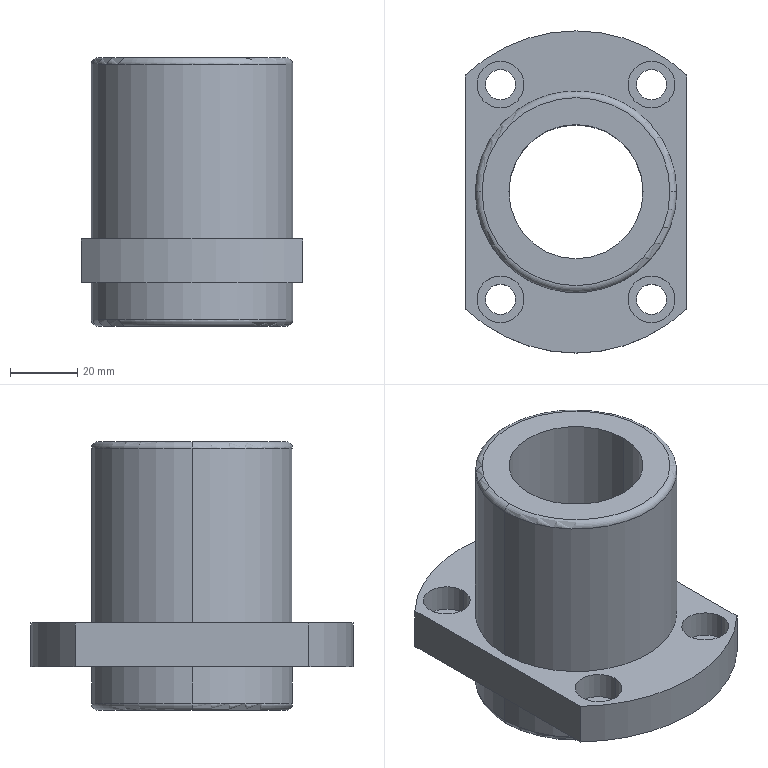Part | SolidWorks | features RevCut 4, ICE 1, LockFeature 1, Revolution 1 | 1 solid | 38 faces | box 66 x 96 x 80 mm | volume 157671 mm3 | cylinder 24 | plane 10 | torus 4 | commonest cylinder face diameters 9 x8 14 x8 60 x4 40 x2 96 x2
STEP:
#1=CARTESIAN_POINT('',(15.5,-32.,4.9));
#2=VERTEX_POINT('',#1);
#3=CARTESIAN_POINT('',(29.5,-32.,4.9));
#4=VERTEX_POINT('',#3);
#5=CARTESIAN_POINT('',(22.5,-32.,4.9));
#6=DIRECTION('',(0.,0.,1.));
#7=DIRECTION('',(1.,0.,0.));
#8=AXIS2_PLACEMENT_3D('',#5,#6,#7);
#9=CIRCLE('',#8,7.);
#10=EDGE_CURVE('',#2,#4,#9,.T.);
#11=ORIENTED_EDGE('',*,*,#10,.F.);
#12=CARTESIAN_POINT('',(15.5,-32.,13.));
#13=VERTEX_POINT('',#12);
#14=CARTESIAN_POINT('',(15.5,-32.,13.));
#15=DIRECTION('',(0.,0.,1.));
#16=VECTOR('',#15,1000.);
#17=LINE('',#14,#16);
#18=EDGE_CURVE('',#2,#13,#17,.T.);
#19=ORIENTED_EDGE('',*,*,#18,.T.);
#20=CARTESIAN_POINT('',(29.5,-32.,13.));
#21=VERTEX_POINT('',#20);
#22=CARTESIAN_POINT('',(22.5,-32.,13.));
#23=DIRECTION('',(0.,0.,1.));
#24=DIRECTION('',(1.,0.,0.));
#25=AXIS2_PLACEMENT_3D('',#22,#23,#24);
#26=CIRCLE('',#25,7.);
#27=EDGE_CURVE('',#13,#21,#26,.T.);
#28=ORIENTED_EDGE('',*,*,#27,.T.);
#29=CARTESIAN_POINT('',(29.5,-32.,13.));
#30=DIRECTION('',(0.,0.,1.));
#31=VECTOR('',#30,1000.);
#32=LINE('',#29,#31);
#33=EDGE_CURVE('',#4,#21,#32,.T.);
#34=ORIENTED_EDGE('',*,*,#33,.F.);
#35=EDGE_LOOP('',(#11,#19,#28,#34));
#36=FACE_OUTER_BOUND('',#35,.T.);
#37=CARTESIAN_POINT('',(22.5,-32.,13.));
#38=DIRECTION('',(0.,0.,1.));
#39=DIRECTION('',(1.,0.,0.));
#40=AXIS2_PLACEMENT_3D('',#37,#38,#39);
#41=CYLINDRICAL_SURFACE('',#40,7.);
#42=ADVANCED_FACE('',(#36),#41,.F.);
#43=CARTESIAN_POINT('',(18.,-32.,0.));
#44=VERTEX_POINT('',#43);
#45=CARTESIAN_POINT('',(27.,-32.,0.));
#46=VERTEX_POINT('',#45);
#47=CARTESIAN_POINT('',(22.5,-32.,0.));
#48=DIRECTION('',(0.,0.,1.));
#49=DIRECTION('',(1.,0.,0.));
#50=AXIS2_PLACEMENT_3D('',#47,#48,#49);
#51=CIRCLE('',#50,4.5);
#52=EDGE_CURVE('',#44,#46,#51,.T.);
#53=ORIENTED_EDGE('',*,*,#52,.F.);
#54=CARTESIAN_POINT('',(18.,-32.,4.9));
#55=VERTEX_POINT('',#54);
#56=CARTESIAN_POINT('',(18.,-32.,13.));
#57=DIRECTION('',(0.,0.,1.));
#58=VECTOR('',#57,1000.);
#59=LINE('',#56,#58);
#60=EDGE_CURVE('',#44,#55,#59,.T.);
#61=ORIENTED_EDGE('',*,*,#60,.T.);
#62=CARTESIAN_POINT('',(27.,-32.,4.9));
#63=VERTEX_POINT('',#62);
#64=CARTESIAN_POINT('',(22.5,-32.,4.9));
#65=DIRECTION('',(0.,0.,1.));
#66=DIRECTION('',(1.,0.,0.));
#67=AXIS2_PLACEMENT_3D('',#64,#65,#66);
#68=CIRCLE('',#67,4.5);
#69=EDGE_CURVE('',#55,#63,#68,.T.);
#70=ORIENTED_EDGE('',*,*,#69,.T.);
#71=CARTESIAN_POINT('',(27.,-32.,13.));
#72=DIRECTION('',(0.,0.,1.));
#73=VECTOR('',#72,1000.);
#74=LINE('',#71,#73);
#75=EDGE_CURVE('',#46,#63,#74,.T.);
#76=ORIENTED_EDGE('',*,*,#75,.F.);
#77=EDGE_LOOP('',(#53,#61,#70,#76));
#78=FACE_OUTER_BOUND('',#77,.T.);
#79=CARTESIAN_POINT('',(22.5,-32.,13.));
#80=DIRECTION('',(0.,0.,1.));
#81=DIRECTION('',(1.,0.,0.));
#82=AXIS2_PLACEMENT_3D('',#79,#80,#81);
#83=CYLINDRICAL_SURFACE('',#82,4.5);
#84=ADVANCED_FACE('',(#78),#83,.F.);
#85=CARTESIAN_POINT('',(27.,32.,4.9));
#86=VERTEX_POINT('',#85);
#87=CARTESIAN_POINT('',(18.,32.,4.9));
#88=VERTEX_POINT('',#87);
#89=CARTESIAN_POINT('',(22.5,32.,4.9));
#90=DIRECTION('',(0.,0.,-1.));
#91=DIRECTION('',(-1.,0.,0.));
#92=AXIS2_PLACEMENT_3D('',#89,#90,#91);
#93=CIRCLE('',#92,4.5);
#94=EDGE_CURVE('',#86,#88,#93,.T.);
#95=ORIENTED_EDGE('',*,*,#94,.F.);
#96=CARTESIAN_POINT('',(27.,32.,0.));
#97=VERTEX_POINT('',#96);
#98=CARTESIAN_POINT('',(27.,32.,0.));
#99=DIRECTION('',(0.,0.,-1.));
#100=VECTOR('',#99,1000.);
#101=LINE('',#98,#100);
#102=EDGE_CURVE('',#86,#97,#101,.T.);
#103=ORIENTED_EDGE('',*,*,#102,.T.);
#104=CARTESIAN_POINT('',(18.,32.,0.));
#105=VERTEX_POINT('',#104);
#106=CARTESIAN_POINT('',(22.5,32.,0.));
#107=DIRECTION('',(0.,0.,-1.));
#108=DIRECTION('',(-1.,0.,0.));
#109=AXIS2_PLACEMENT_3D('',#106,#107,#108);
#110=CIRCLE('',#109,4.5);
#111=EDGE_CURVE('',#97,#105,#110,.T.);
#112=ORIENTED_EDGE('',*,*,#111,.T.);
#113=CARTESIAN_POINT('',(18.,32.,0.));
#114=DIRECTION('',(0.,0.,-1.));
#115=VECTOR('',#114,1000.);
#116=LINE('',#113,#115);
#117=EDGE_CURVE('',#88,#105,#116,.T.);
#118=ORIENTED_EDGE('',*,*,#117,.F.);
#119=EDGE_LOOP('',(#95,#103,#112,#118));
#120=FACE_OUTER_BOUND('',#119,.T.);
#121=CARTESIAN_POINT('',(22.5,32.,0.));
#122=DIRECTION('',(0.,0.,-1.));
#123=DIRECTION('',(-1.,0.,0.));
#124=AXIS2_PLACEMENT_3D('',#121,#122,#123);
#125=CYLINDRICAL_SURFACE('',#124,4.5);
#126=ADVANCED_FACE('',(#120),#125,.F.);
#127=CARTESIAN_POINT('',(29.5,32.,13.));
#128=VERTEX_POINT('',#127);
#129=CARTESIAN_POINT('',(15.5,32.,13.));
#130=VERTEX_POINT('',#129);
#131=CARTESIAN_POINT('',(22.5,32.,13.));
#132=DIRECTION('',(0.,0.,-1.));
#133=DIRECTION('',(-1.,0.,0.));
#134=AXIS2_PLACEMENT_3D('',#131,#132,#133);
#135=CIRCLE('',#134,7.);
#136=EDGE_CURVE('',#128,#130,#135,.T.);
#137=ORIENTED_EDGE('',*,*,#136,.F.);
#138=CARTESIAN_POINT('',(29.5,32.,4.9));
#139=VERTEX_POINT('',#138);
#140=CARTESIAN_POINT('',(29.5,32.,0.));
#141=DIRECTION('',(0.,0.,-1.));
#142=VECTOR('',#141,1000.);
#143=LINE('',#140,#142);
#144=EDGE_CURVE('',#128,#139,#143,.T.);
#145=ORIENTED_EDGE('',*,*,#144,.T.);
#146=CARTESIAN_POINT('',(15.5,32.,4.9));
#147=VERTEX_POINT('',#146);
#148=CARTESIAN_POINT('',(22.5,32.,4.9));
#149=DIRECTION('',(0.,0.,-1.));
#150=DIRECTION('',(-1.,0.,0.));
#151=AXIS2_PLACEMENT_3D('',#148,#149,#150);
#152=CIRCLE('',#151,7.);
#153=EDGE_CURVE('',#139,#147,#152,.T.);
#154=ORIENTED_EDGE('',*,*,#153,.T.);
#155=CARTESIAN_POINT('',(15.5,32.,0.));
#156=DIRECTION('',(0.,0.,-1.));
#157=VECTOR('',#156,1000.);
#158=LINE('',#155,#157);
#159=EDGE_CURVE('',#130,#147,#158,.T.);
#160=ORIENTED_EDGE('',*,*,#159,.F.);
#161=EDGE_LOOP('',(#137,#145,#154,#160));
#162=FACE_OUTER_BOUND('',#161,.T.);
#163=CARTESIAN_POINT('',(22.5,32.,0.));
#164=DIRECTION('',(0.,0.,-1.));
#165=DIRECTION('',(-1.,0.,0.));
#166=AXIS2_PLACEMENT_3D('',#163,#164,#165);
#167=CYLINDRICAL_SURFACE('',#166,7.);
#168=ADVANCED_FACE('',(#162),#167,.F.);
#169=CARTESIAN_POINT('',(-29.5,-32.,4.9));
#170=VERTEX_POINT('',#169);
#171=CARTESIAN_POINT('',(-15.5,-32.,4.9));
#172=VERTEX_POINT('',#171);
#173=CARTESIAN_POINT('',(-22.5,-32.,4.9));
#174=DIRECTION('',(0.,0.,1.));
#175=DIRECTION('',(1.,0.,0.));
#176=AXIS2_PLACEMENT_3D('',#173,#174,#175);
#177=CIRCLE('',#176,7.);
#178=EDGE_CURVE('',#170,#172,#177,.T.);
#179=ORIENTED_EDGE('',*,*,#178,.F.);
#180=CARTESIAN_POINT('',(-29.5,-32.,13.));
#181=VERTEX_POINT('',#180);
#182=CARTESIAN_POINT('',(-29.5,-32.,13.));
#183=DIRECTION('',(0.,0.,1.));
#184=VECTOR('',#183,1000.);
#185=LINE('',#182,#184);
#186=EDGE_CURVE('',#170,#181,#185,.T.);
#187=ORIENTED_EDGE('',*,*,#186,.T.);
#188=CARTESIAN_POINT('',(-15.5,-32.,13.));
#189=VERTEX_POINT('',#188);
#190=CARTESIAN_POINT('',(-22.5,-32.,13.));
#191=DIRECTION('',(0.,0.,1.));
#192=DIRECTION('',(1.,0.,0.));
#193=AXIS2_PLACEMENT_3D('',#190,#191,#192);
#194=CIRCLE('',#193,7.);
#195=EDGE_CURVE('',#181,#189,#194,.T.);
#196=ORIENTED_EDGE('',*,*,#195,.T.);
#197=CARTESIAN_POINT('',(-15.5,-32.,13.));
#198=DIRECTION('',(0.,0.,1.));
#199=VECTOR('',#198,1000.);
#200=LINE('',#197,#199);
#201=EDGE_CURVE('',#172,#189,#200,.T.);
#202=ORIENTED_EDGE('',*,*,#201,.F.);
#203=EDGE_LOOP('',(#179,#187,#196,#202));
#204=FACE_OUTER_BOUND('',#203,.T.);
#205=CARTESIAN_POINT('',(-22.5,-32.,13.));
#206=DIRECTION('',(0.,0.,1.));
#207=DIRECTION('',(1.,0.,0.));
#208=AXIS2_PLACEMENT_3D('',#205,#206,#207);
#209=CYLINDRICAL_SURFACE('',#208,7.);
#210=ADVANCED_FACE('',(#204),#209,.F.);
#211=CARTESIAN_POINT('',(-27.,-32.,0.));
#212=VERTEX_POINT('',#211);
#213=CARTESIAN_POINT('',(-18.,-32.,0.));
#214=VERTEX_POINT('',#213);
#215=CARTESIAN_POINT('',(-22.5,-32.,0.));
#216=DIRECTION('',(0.,0.,1.));
#217=DIRECTION('',(1.,0.,0.));
#218=AXIS2_PLACEMENT_3D('',#215,#216,#217);
#219=CIRCLE('',#218,4.5);
#220=EDGE_CURVE('',#212,#214,#219,.T.);
#221=ORIENTED_EDGE('',*,*,#220,.F.);
#222=CARTESIAN_POINT('',(-27.,-32.,4.9));
#223=VERTEX_POINT('',#222);
#224=CARTESIAN_POINT('',(-27.,-32.,13.));
#225=DIRECTION('',(0.,0.,1.));
#226=VECTOR('',#225,1000.);
#227=LINE('',#224,#226);
#228=EDGE_CURVE('',#212,#223,#227,.T.);
#229=ORIENTED_EDGE('',*,*,#228,.T.);
#230=CARTESIAN_POINT('',(-18.,-32.,4.9));
#231=VERTEX_POINT('',#230);
#232=CARTESIAN_POINT('',(-22.5,-32.,4.9));
#233=DIRECTION('',(0.,0.,1.));
#234=DIRECTION('',(1.,0.,0.));
#235=AXIS2_PLACEMENT_3D('',#232,#233,#234);
#236=CIRCLE('',#235,4.5);
#237=EDGE_CURVE('',#223,#231,#236,.T.);
#238=ORIENTED_EDGE('',*,*,#237,.T.);
#239=CARTESIAN_POINT('',(-18.,-32.,13.));
#240=DIRECTION('',(0.,0.,1.));
#241=VECTOR('',#240,1000.);
#242=LINE('',#239,#241);
#243=EDGE_CURVE('',#214,#231,#242,.T.);
#244=ORIENTED_EDGE('',*,*,#243,.F.);
#245=EDGE_LOOP('',(#221,#229,#238,#244));
#246=FACE_OUTER_BOUND('',#245,.T.);
#247=CARTESIAN_POINT('',(-22.5,-32.,13.));
#248=DIRECTION('',(0.,0.,1.));
#249=DIRECTION('',(1.,0.,0.));
#250=AXIS2_PLACEMENT_3D('',#247,#248,#249);
#251=CYLINDRICAL_SURFACE('',#250,4.5);
#252=ADVANCED_FACE('',(#246),#251,.F.);
#253=CARTESIAN_POINT('',(-18.,32.,4.9));
#254=VERTEX_POINT('',#253);
#255=CARTESIAN_POINT('',(-27.,32.,4.9));
#256=VERTEX_POINT('',#255);
#257=CARTESIAN_POINT('',(-22.5,32.,4.9));
#258=DIRECTION('',(0.,0.,-1.));
#259=DIRECTION('',(-1.,0.,0.));
#260=AXIS2_PLACEMENT_3D('',#257,#258,#259);
#261=CIRCLE('',#260,4.5);
#262=EDGE_CURVE('',#254,#256,#261,.T.);
#263=ORIENTED_EDGE('',*,*,#262,.F.);
#264=CARTESIAN_POINT('',(-18.,32.,0.));
#265=VERTEX_POINT('',#264);
#266=CARTESIAN_POINT('',(-18.,32.,0.));
#267=DIRECTION('',(0.,0.,-1.));
#268=VECTOR('',#267,1000.);
#269=LINE('',#266,#268);
#270=EDGE_CURVE('',#254,#265,#269,.T.);
#271=ORIENTED_EDGE('',*,*,#270,.T.);
#272=CARTESIAN_POINT('',(-27.,32.,0.));
#273=VERTEX_POINT('',#272);
#274=CARTESIAN_POINT('',(-22.5,32.,0.));
#275=DIRECTION('',(0.,0.,-1.));
#276=DIRECTION('',(-1.,0.,0.));
#277=AXIS2_PLACEMENT_3D('',#274,#275,#276);
#278=CIRCLE('',#277,4.5);
#279=EDGE_CURVE('',#265,#273,#278,.T.);
#280=ORIENTED_EDGE('',*,*,#279,.T.);
#281=CARTESIAN_POINT('',(-27.,32.,0.));
#282=DIRECTION('',(0.,0.,-1.));
#283=VECTOR('',#282,1000.);
#284=LINE('',#281,#283);
#285=EDGE_CURVE('',#256,#273,#284,.T.);
#286=ORIENTED_EDGE('',*,*,#285,.F.);
#287=EDGE_LOOP('',(#263,#271,#280,#286));
#288=FACE_OUTER_BOUND('',#287,.T.);
#289=CARTESIAN_POINT('',(-22.5,32.,0.));
#290=DIRECTION('',(0.,0.,-1.));
#291=DIRECTION('',(-1.,0.,0.));
#292=AXIS2_PLACEMENT_3D('',#289,#290,#291);
#293=CYLINDRICAL_SURFACE('',#292,4.5);
#294=ADVANCED_FACE('',(#288),#293,.F.);
#295=CARTESIAN_POINT('',(-15.5,32.,13.));
#296=VERTEX_POINT('',#295);
#297=CARTESIAN_POINT('',(-29.5,32.,13.));
#298=VERTEX_POINT('',#297);
#299=CARTESIAN_POINT('',(-22.5,32.,13.));
#300=DIRECTION('',(0.,0.,-1.));
#301=DIRECTION('',(-1.,0.,0.));
#302=AXIS2_PLACEMENT_3D('',#299,#300,#301);
#303=CIRCLE('',#302,7.);
#304=EDGE_CURVE('',#296,#298,#303,.T.);
#305=ORIENTED_EDGE('',*,*,#304,.F.);
#306=CARTESIAN_POINT('',(-15.5,32.,4.9));
#307=VERTEX_POINT('',#306);
#308=CARTESIAN_POINT('',(-15.5,32.,0.));
#309=DIRECTION('',(0.,0.,-1.));
#310=VECTOR('',#309,1000.);
#311=LINE('',#308,#310);
#312=EDGE_CURVE('',#296,#307,#311,.T.);
#313=ORIENTED_EDGE('',*,*,#312,.T.);
#314=CARTESIAN_POINT('',(-29.5,32.,4.9));
#315=VERTEX_POINT('',#314);
#316=CARTESIAN_POINT('',(-22.5,32.,4.9));
#317=DIRECTION('',(0.,0.,-1.));
#318=DIRECTION('',(-1.,0.,0.));
#319=AXIS2_PLACEMENT_3D('',#316,#317,#318);
#320=CIRCLE('',#319,7.);
#321=EDGE_CURVE('',#307,#315,#320,.T.);
#322=ORIENTED_EDGE('',*,*,#321,.T.);
#323=CARTESIAN_POINT('',(-29.5,32.,0.));
#324=DIRECTION('',(0.,0.,-1.));
#325=VECTOR('',#324,1000.);
#326=LINE('',#323,#325);
#327=EDGE_CURVE('',#298,#315,#326,.T.);
#328=ORIENTED_EDGE('',*,*,#327,.F.);
#329=EDGE_LOOP('',(#305,#313,#322,#328));
#330=FACE_OUTER_BOUND('',#329,.T.);
#331=CARTESIAN_POINT('',(-22.5,32.,0.));
#332=DIRECTION('',(0.,0.,-1.));
#333=DIRECTION('',(-1.,0.,0.));
#334=AXIS2_PLACEMENT_3D('',#331,#332,#333);
#335=CYLINDRICAL_SURFACE('',#334,7.);
#336=ADVANCED_FACE('',(#330),#335,.F.);
#337=CARTESIAN_POINT('',(-30.,0.,65.));
#338=VERTEX_POINT('',#337);
#339=CARTESIAN_POINT('',(30.,0.,65.));
#340=VERTEX_POINT('',#339);
#341=CARTESIAN_POINT('',(0.,0.,65.));
#342=DIRECTION('',(0.,0.,-1.));
#343=DIRECTION('',(-1.,0.,0.));
#344=AXIS2_PLACEMENT_3D('',#341,#342,#343);
#345=CIRCLE('',#344,30.);
#346=EDGE_CURVE('',#338,#340,#345,.T.);
#347=ORIENTED_EDGE('',*,*,#346,.T.);
#348=CARTESIAN_POINT('',(30.,0.,13.));
#349=VERTEX_POINT('',#348);
#350=CARTESIAN_POINT('',(30.,0.,-13.));
#351=DIRECTION('',(0.,0.,-1.));
#352=VECTOR('',#351,1000.);
#353=LINE('',#350,#352);
#354=EDGE_CURVE('',#340,#349,#353,.T.);
#355=ORIENTED_EDGE('',*,*,#354,.T.);
#356=CARTESIAN_POINT('',(-30.,0.,13.));
#357=VERTEX_POINT('',#356);
#358=CARTESIAN_POINT('',(0.,0.,13.));
#359=DIRECTION('',(0.,0.,-1.));
#360=DIRECTION('',(1.,0.,0.));
#361=AXIS2_PLACEMENT_3D('',#358,#359,#360);
#362=CIRCLE('',#361,30.);
#363=EDGE_CURVE('',#357,#349,#362,.T.);
#364=ORIENTED_EDGE('',*,*,#363,.F.);
#365=CARTESIAN_POINT('',(-30.,0.,-13.));
#366=DIRECTION('',(0.,0.,-1.));
#367=VECTOR('',#366,1000.);
#368=LINE('',#365,#367);
#369=EDGE_CURVE('',#338,#357,#368,.T.);
#370=ORIENTED_EDGE('',*,*,#369,.F.);
#371=EDGE_LOOP('',(#347,#355,#364,#370));
#372=FACE_OUTER_BOUND('',#371,.T.);
#373=CARTESIAN_POINT('',(0.,0.,-13.));
#374=DIRECTION('',(0.,0.,-1.));
#375=DIRECTION('',(-1.,0.,0.));
#376=AXIS2_PLACEMENT_3D('',#373,#374,#375);
#377=CYLINDRICAL_SURFACE('',#376,30.);
#378=ADVANCED_FACE('',(#372),#377,.T.);
#379=CARTESIAN_POINT('',(-30.,0.,-11.));
#380=VERTEX_POINT('',#379);
#381=CARTESIAN_POINT('',(30.,0.,-11.));
#382=VERTEX_POINT('',#381);
#383=CARTESIAN_POINT('',(0.,0.,-11.));
#384=DIRECTION('',(0.,0.,-1.));
#385=DIRECTION('',(-1.,0.,0.));
#386=AXIS2_PLACEMENT_3D('',#383,#384,#385);
#387=CIRCLE('',#386,30.);
#388=EDGE_CURVE('',#380,#382,#387,.T.);
#389=ORIENTED_EDGE('',*,*,#388,.T.);
#390=CARTESIAN_POINT('',(28.,0.,-13.));
#391=VERTEX_POINT('',#390);
#392=CARTESIAN_POINT('',(28.,0.,-11.));
#393=DIRECTION('',(0.,1.,0.));
#394=DIRECTION('',(-1.,0.,0.));
#395=AXIS2_PLACEMENT_3D('',#392,#393,#394);
#396=CIRCLE('',#395,2.);
#397=EDGE_CURVE('',#382,#391,#396,.T.);
#398=ORIENTED_EDGE('',*,*,#397,.T.);
#399=CARTESIAN_POINT('',(-28.,0.,-13.));
#400=VERTEX_POINT('',#399);
#401=CARTESIAN_POINT('',(0.,0.,-13.));
#402=DIRECTION('',(0.,0.,-1.));
#403=DIRECTION('',(-1.,0.,0.));
#404=AXIS2_PLACEMENT_3D('',#401,#402,#403);
#405=CIRCLE('',#404,28.);
#406=EDGE_CURVE('',#400,#391,#405,.T.);
#407=ORIENTED_EDGE('',*,*,#406,.F.);
#408=CARTESIAN_POINT('',(-28.,0.,-11.));
#409=DIRECTION('',(0.,-1.,0.));
#410=DIRECTION('',(0.,0.,-1.));
#411=AXIS2_PLACEMENT_3D('',#408,#409,#410);
#412=CIRCLE('',#411,2.);
#413=EDGE_CURVE('',#380,#400,#412,.T.);
#414=ORIENTED_EDGE('',*,*,#413,.F.);
#415=EDGE_LOOP('',(#389,#398,#407,#414));
#416=FACE_OUTER_BOUND('',#415,.T.);
#417=CARTESIAN_POINT('',(0.,0.,-11.));
#418=DIRECTION('',(0.,0.,-1.));
#419=DIRECTION('',(-1.,0.,0.));
#420=AXIS2_PLACEMENT_3D('',#417,#418,#419);
#421=TOROIDAL_SURFACE('',#420,28.,2.);
#422=ADVANCED_FACE('',(#416),#421,.T.);
#423=CARTESIAN_POINT('',(20.,0.,67.));
#424=VERTEX_POINT('',#423);
#425=CARTESIAN_POINT('',(-20.,0.,67.));
#426=VERTEX_POINT('',#425);
#427=CARTESIAN_POINT('',(0.,0.,67.));
#428=DIRECTION('',(0.,0.,-1.));
#429=DIRECTION('',(-1.,0.,0.));
#430=AXIS2_PLACEMENT_3D('',#427,#428,#429);
#431=CIRCLE('',#430,20.);
#432=EDGE_CURVE('',#424,#426,#431,.T.);
#433=ORIENTED_EDGE('',*,*,#432,.F.);
#434=CARTESIAN_POINT('',(20.,0.,-13.));
#435=VERTEX_POINT('',#434);
#436=CARTESIAN_POINT('',(20.,0.,-13.));
#437=DIRECTION('',(0.,0.,-1.));
#438=VECTOR('',#437,1000.);
#439=LINE('',#436,#438);
#440=EDGE_CURVE('',#424,#435,#439,.T.);
#441=ORIENTED_EDGE('',*,*,#440,.T.);
#442=CARTESIAN_POINT('',(-20.,0.,-13.));
#443=VERTEX_POINT('',#442);
#444=CARTESIAN_POINT('',(0.,0.,-13.));
#445=DIRECTION('',(0.,0.,-1.));
#446=DIRECTION('',(-1.,0.,0.));
#447=AXIS2_PLACEMENT_3D('',#444,#445,#446);
#448=CIRCLE('',#447,20.);
#449=EDGE_CURVE('',#435,#443,#448,.T.);
#450=ORIENTED_EDGE('',*,*,#449,.T.);
#451=CARTESIAN_POINT('',(-20.,0.,-13.));
#452=DIRECTION('',(0.,0.,-1.));
#453=VECTOR('',#452,1000.);
#454=LINE('',#451,#453);
#455=EDGE_CURVE('',#426,#443,#454,.T.);
#456=ORIENTED_EDGE('',*,*,#455,.F.);
#457=EDGE_LOOP('',(#433,#441,#450,#456));
#458=FACE_OUTER_BOUND('',#457,.T.);
#459=CARTESIAN_POINT('',(0.,0.,-13.));
#460=DIRECTION('',(0.,0.,-1.));
#461=DIRECTION('',(-1.,0.,0.));
#462=AXIS2_PLACEMENT_3D('',#459,#460,#461);
#463=CYLINDRICAL_SURFACE('',#462,20.);
#464=ADVANCED_FACE('',(#458),#463,.F.);
#465=CARTESIAN_POINT('',(-28.,0.,67.));
#466=VERTEX_POINT('',#465);
#467=CARTESIAN_POINT('',(28.,0.,67.));
#468=VERTEX_POINT('',#467);
#469=CARTESIAN_POINT('',(0.,0.,67.));
#470=DIRECTION('',(0.,0.,-1.));
#471=DIRECTION('',(-1.,0.,0.));
#472=AXIS2_PLACEMENT_3D('',#469,#470,#471);
#473=CIRCLE('',#472,28.);
#474=EDGE_CURVE('',#466,#468,#473,.T.);
#475=ORIENTED_EDGE('',*,*,#474,.T.);
#476=CARTESIAN_POINT('',(28.,0.,65.));
#477=DIRECTION('',(0.,1.,0.));
#478=DIRECTION('',(-1.,0.,0.));
#479=AXIS2_PLACEMENT_3D('',#476,#477,#478);
#480=CIRCLE('',#479,2.);
#481=EDGE_CURVE('',#468,#340,#480,.T.);
#482=ORIENTED_EDGE('',*,*,#481,.T.);
#483=ORIENTED_EDGE('',*,*,#346,.F.);
#484=CARTESIAN_POINT('',(-28.,0.,65.));
#485=DIRECTION('',(0.,-1.,0.));
#486=DIRECTION('',(0.,0.,-1.));
#487=AXIS2_PLACEMENT_3D('',#484,#485,#486);
#488=CIRCLE('',#487,2.);
#489=EDGE_CURVE('',#466,#338,#488,.T.);
#490=ORIENTED_EDGE('',*,*,#489,.F.);
#491=EDGE_LOOP('',(#475,#482,#483,#490));
#492=FACE_OUTER_BOUND('',#491,.T.);
#493=CARTESIAN_POINT('',(0.,0.,65.));
#494=DIRECTION('',(0.,0.,-1.));
#495=DIRECTION('',(-1.,0.,0.));
#496=AXIS2_PLACEMENT_3D('',#493,#494,#495);
#497=TOROIDAL_SURFACE('',#496,28.,2.);
#498=ADVANCED_FACE('',(#492),#497,.T.);
#499=CARTESIAN_POINT('',(30.,0.,0.));
#500=VERTEX_POINT('',#499);
#501=CARTESIAN_POINT('',(-30.,0.,0.));
#502=VERTEX_POINT('',#501);
#503=CARTESIAN_POINT('',(0.,0.,0.));
#504=DIRECTION('',(0.,0.,1.));
#505=DIRECTION('',(1.,0.,0.));
#506=AXIS2_PLACEMENT_3D('',#503,#504,#505);
#507=CIRCLE('',#506,30.);
#508=EDGE_CURVE('',#500,#502,#507,.T.);
#509=ORIENTED_EDGE('',*,*,#508,.F.);
#510=CARTESIAN_POINT('',(30.,0.,-13.));
#511=DIRECTION('',(0.,0.,-1.));
#512=VECTOR('',#511,1000.);
#513=LINE('',#510,#512);
#514=EDGE_CURVE('',#500,#382,#513,.T.);
#515=ORIENTED_EDGE('',*,*,#514,.T.);
#516=ORIENTED_EDGE('',*,*,#388,.F.);
#517=CARTESIAN_POINT('',(-30.,0.,-13.));
#518=DIRECTION('',(0.,0.,-1.));
#519=VECTOR('',#518,1000.);
#520=LINE('',#517,#519);
#521=EDGE_CURVE('',#502,#380,#520,.T.);
#522=ORIENTED_EDGE('',*,*,#521,.F.);
#523=EDGE_LOOP('',(#509,#515,#516,#522));
#524=FACE_OUTER_BOUND('',#523,.T.);
#525=CARTESIAN_POINT('',(0.,0.,-13.));
#526=DIRECTION('',(0.,0.,-1.));
#527=DIRECTION('',(-1.,0.,0.));
#528=AXIS2_PLACEMENT_3D('',#525,#526,#527);
#529=CYLINDRICAL_SURFACE('',#528,30.);
#530=ADVANCED_FACE('',(#524),#529,.T.);
#531=ORIENTED_EDGE('',*,*,#514,.F.);
#532=CARTESIAN_POINT('',(0.,0.,0.));
#533=DIRECTION('',(0.,0.,1.));
#534=DIRECTION('',(1.,0.,0.));
#535=AXIS2_PLACEMENT_3D('',#532,#533,#534);
#536=CIRCLE('',#535,30.);
#537=EDGE_CURVE('',#502,#500,#536,.T.);
#538=ORIENTED_EDGE('',*,*,#537,.F.);
#539=ORIENTED_EDGE('',*,*,#521,.T.);
#540=CARTESIAN_POINT('',(0.,0.,-11.));
#541=DIRECTION('',(0.,0.,-1.));
#542=DIRECTION('',(-1.,0.,0.));
#543=AXIS2_PLACEMENT_3D('',#540,#541,#542);
#544=CIRCLE('',#543,30.);
#545=EDGE_CURVE('',#382,#380,#544,.T.);
#546=ORIENTED_EDGE('',*,*,#545,.F.);
#547=EDGE_LOOP('',(#531,#538,#539,#546));
#548=FACE_OUTER_BOUND('',#547,.T.);
#549=CARTESIAN_POINT('',(0.,0.,-13.));
#550=DIRECTION('',(0.,0.,-1.));
#551=DIRECTION('',(-1.,0.,0.));
#552=AXIS2_PLACEMENT_3D('',#549,#550,#551);
#553=CYLINDRICAL_SURFACE('',#552,30.);
#554=ADVANCED_FACE('',(#548),#553,.T.);
#555=ORIENTED_EDGE('',*,*,#481,.F.);
#556=CARTESIAN_POINT('',(0.,0.,67.));
#557=DIRECTION('',(0.,0.,-1.));
#558=DIRECTION('',(-1.,0.,0.));
#559=AXIS2_PLACEMENT_3D('',#556,#557,#558);
#560=CIRCLE('',#559,28.);
#561=EDGE_CURVE('',#468,#466,#560,.T.);
#562=ORIENTED_EDGE('',*,*,#561,.T.);
#563=ORIENTED_EDGE('',*,*,#489,.T.);
#564=CARTESIAN_POINT('',(0.,0.,65.));
#565=DIRECTION('',(0.,0.,-1.));
#566=DIRECTION('',(-1.,0.,0.));
#567=AXIS2_PLACEMENT_3D('',#564,#565,#566);
#568=CIRCLE('',#567,30.);
#569=EDGE_CURVE('',#340,#338,#568,.T.);
#570=ORIENTED_EDGE('',*,*,#569,.F.);
#571=EDGE_LOOP('',(#555,#562,#563,#570));
#572=FACE_OUTER_BOUND('',#571,.T.);
#573=CARTESIAN_POINT('',(0.,0.,65.));
#574=DIRECTION('',(0.,0.,-1.));
#575=DIRECTION('',(-1.,0.,0.));
#576=AXIS2_PLACEMENT_3D('',#573,#574,#575);
#577=TOROIDAL_SURFACE('',#576,28.,2.);
#578=ADVANCED_FACE('',(#572),#577,.T.);
#579=CARTESIAN_POINT('',(0.,0.,67.));
#580=DIRECTION('',(0.,0.,-1.));
#581=DIRECTION('',(-1.,0.,0.));
#582=AXIS2_PLACEMENT_3D('',#579,#580,#581);
#583=CIRCLE('',#582,20.);
#584=EDGE_CURVE('',#426,#424,#583,.T.);
#585=ORIENTED_EDGE('',*,*,#584,.T.);
#586=ORIENTED_EDGE('',*,*,#432,.T.);
#587=EDGE_LOOP('',(#585,#586));
#588=FACE_BOUND('',#587,.T.);
#589=ORIENTED_EDGE('',*,*,#474,.F.);
#590=ORIENTED_EDGE('',*,*,#561,.F.);
#591=EDGE_LOOP('',(#589,#590));
#592=FACE_OUTER_BOUND('',#591,.T.);
#593=CARTESIAN_POINT('',(0.,28.,67.));
#594=DIRECTION('',(0.,0.,1.));
#595=DIRECTION('',(1.,0.,0.));
#596=AXIS2_PLACEMENT_3D('',#593,#594,#595);
#597=PLANE('',#596);
#598=ADVANCED_FACE('',(#588,#592),#597,.T.);
#599=ORIENTED_EDGE('',*,*,#440,.F.);
#600=ORIENTED_EDGE('',*,*,#584,.F.);
#601=ORIENTED_EDGE('',*,*,#455,.T.);
#602=CARTESIAN_POINT('',(0.,0.,-13.));
#603=DIRECTION('',(0.,0.,-1.));
#604=DIRECTION('',(-1.,0.,0.));
#605=AXIS2_PLACEMENT_3D('',#602,#603,#604);
#606=CIRCLE('',#605,20.);
#607=EDGE_CURVE('',#443,#435,#606,.T.);
#608=ORIENTED_EDGE('',*,*,#607,.T.);
#609=EDGE_LOOP('',(#599,#600,#601,#608));
#610=FACE_OUTER_BOUND('',#609,.T.);
#611=CARTESIAN_POINT('',(0.,0.,-13.));
#612=DIRECTION('',(0.,0.,-1.));
#613=DIRECTION('',(-1.,0.,0.));
#614=AXIS2_PLACEMENT_3D('',#611,#612,#613);
#615=CYLINDRICAL_SURFACE('',#614,20.);
#616=ADVANCED_FACE('',(#610),#615,.F.);
#617=ORIENTED_EDGE('',*,*,#406,.T.);
#618=CARTESIAN_POINT('',(0.,0.,-13.));
#619=DIRECTION('',(0.,0.,-1.));
#620=DIRECTION('',(-1.,0.,0.));
#621=AXIS2_PLACEMENT_3D('',#618,#619,#620);
#622=CIRCLE('',#621,28.);
#623=EDGE_CURVE('',#391,#400,#622,.T.);
#624=ORIENTED_EDGE('',*,*,#623,.T.);
#625=EDGE_LOOP('',(#617,#624));
#626=FACE_OUTER_BOUND('',#625,.T.);
#627=ORIENTED_EDGE('',*,*,#607,.F.);
#628=ORIENTED_EDGE('',*,*,#449,.F.);
#629=EDGE_LOOP('',(#627,#628));
#630=FACE_BOUND('',#629,.T.);
#631=CARTESIAN_POINT('',(0.,20.,-13.));
#632=DIRECTION('',(0.,0.,-1.));
#633=DIRECTION('',(-1.,0.,0.));
#634=AXIS2_PLACEMENT_3D('',#631,#632,#633);
#635=PLANE('',#634);
#636=ADVANCED_FACE('',(#626,#630),#635,.T.);
#637=ORIENTED_EDGE('',*,*,#397,.F.);
#638=ORIENTED_EDGE('',*,*,#545,.T.);
#639=ORIENTED_EDGE('',*,*,#413,.T.);
#640=ORIENTED_EDGE('',*,*,#623,.F.);
#641=EDGE_LOOP('',(#637,#638,#639,#640));
#642=FACE_OUTER_BOUND('',#641,.T.);
#643=CARTESIAN_POINT('',(0.,0.,-11.));
#644=DIRECTION('',(0.,0.,-1.));
#645=DIRECTION('',(-1.,0.,0.));
#646=AXIS2_PLACEMENT_3D('',#643,#644,#645);
#647=TOROIDAL_SURFACE('',#646,28.,2.);
#648=ADVANCED_FACE('',(#642),#647,.T.);
#649=ORIENTED_EDGE('',*,*,#354,.F.);
#650=ORIENTED_EDGE('',*,*,#569,.T.);
#651=ORIENTED_EDGE('',*,*,#369,.T.);
#652=CARTESIAN_POINT('',(0.,0.,13.));
#653=DIRECTION('',(0.,0.,-1.));
#654=DIRECTION('',(1.,0.,0.));
#655=AXIS2_PLACEMENT_3D('',#652,#653,#654);
#656=CIRCLE('',#655,30.);
#657=EDGE_CURVE('',#349,#357,#656,.T.);
#658=ORIENTED_EDGE('',*,*,#657,.F.);
#659=EDGE_LOOP('',(#649,#650,#651,#658));
#660=FACE_OUTER_BOUND('',#659,.T.);
#661=CARTESIAN_POINT('',(0.,0.,-13.));
#662=DIRECTION('',(0.,0.,-1.));
#663=DIRECTION('',(-1.,0.,0.));
#664=AXIS2_PLACEMENT_3D('',#661,#662,#663);
#665=CYLINDRICAL_SURFACE('',#664,30.);
#666=ADVANCED_FACE('',(#660),#665,.T.);
#667=CARTESIAN_POINT('',(22.5,-32.,13.));
#668=DIRECTION('',(0.,0.,1.));
#669=DIRECTION('',(1.,0.,0.));
#670=AXIS2_PLACEMENT_3D('',#667,#668,#669);
#671=CIRCLE('',#670,7.);
#672=EDGE_CURVE('',#21,#13,#671,.T.);
#673=ORIENTED_EDGE('',*,*,#672,.F.);
#674=ORIENTED_EDGE('',*,*,#27,.F.);
#675=EDGE_LOOP('',(#673,#674));
#676=FACE_BOUND('',#675,.T.);
#677=CARTESIAN_POINT('',(22.5,32.,13.));
#678=DIRECTION('',(0.,0.,-1.));
#679=DIRECTION('',(-1.,0.,0.));
#680=AXIS2_PLACEMENT_3D('',#677,#678,#679);
#681=CIRCLE('',#680,7.);
#682=EDGE_CURVE('',#130,#128,#681,.T.);
#683=ORIENTED_EDGE('',*,*,#682,.T.);
#684=ORIENTED_EDGE('',*,*,#136,.T.);
#685=EDGE_LOOP('',(#683,#684));
#686=FACE_BOUND('',#685,.T.);
#687=CARTESIAN_POINT('',(-22.5,-32.,13.));
#688=DIRECTION('',(0.,0.,1.));
#689=DIRECTION('',(1.,0.,0.));
#690=AXIS2_PLACEMENT_3D('',#687,#688,#689);
#691=CIRCLE('',#690,7.);
#692=EDGE_CURVE('',#189,#181,#691,.T.);
#693=ORIENTED_EDGE('',*,*,#692,.F.);
#694=ORIENTED_EDGE('',*,*,#195,.F.);
#695=EDGE_LOOP('',(#693,#694));
#696=FACE_BOUND('',#695,.T.);
#697=CARTESIAN_POINT('',(-22.5,32.,13.));
#698=DIRECTION('',(0.,0.,-1.));
#699=DIRECTION('',(-1.,0.,0.));
#700=AXIS2_PLACEMENT_3D('',#697,#698,#699);
#701=CIRCLE('',#700,7.);
#702=EDGE_CURVE('',#298,#296,#701,.T.);
#703=ORIENTED_EDGE('',*,*,#702,.T.);
#704=ORIENTED_EDGE('',*,*,#304,.T.);
#705=EDGE_LOOP('',(#703,#704));
#706=FACE_BOUND('',#705,.T.);
#707=CARTESIAN_POINT('',(33.,34.857,13.));
#708=VERTEX_POINT('',#707);
#709=CARTESIAN_POINT('',(-33.,34.857,13.));
#710=VERTEX_POINT('',#709);
#711=CARTESIAN_POINT('',(0.,0.,13.));
#712=DIRECTION('',(0.,0.,1.));
#713=DIRECTION('',(1.,0.,0.));
#714=AXIS2_PLACEMENT_3D('',#711,#712,#713);
#715=CIRCLE('',#714,48.);
#716=EDGE_CURVE('',#708,#710,#715,.T.);
#717=ORIENTED_EDGE('',*,*,#716,.T.);
#718=CARTESIAN_POINT('',(-33.,-34.857,13.));
#719=VERTEX_POINT('',#718);
#720=CARTESIAN_POINT('',(-33.,34.857,13.));
#721=DIRECTION('',(0.,-1.,0.));
#722=VECTOR('',#721,1000.);
#723=LINE('',#720,#722);
#724=EDGE_CURVE('',#710,#719,#723,.T.);
#725=ORIENTED_EDGE('',*,*,#724,.T.);
#726=CARTESIAN_POINT('',(33.,-34.857,13.));
#727=VERTEX_POINT('',#726);
#728=CARTESIAN_POINT('',(0.,0.,13.));
#729=DIRECTION('',(0.,0.,1.));
#730=DIRECTION('',(1.,0.,0.));
#731=AXIS2_PLACEMENT_3D('',#728,#729,#730);
#732=CIRCLE('',#731,48.);
#733=EDGE_CURVE('',#719,#727,#732,.T.);
#734=ORIENTED_EDGE('',*,*,#733,.T.);
#735=CARTESIAN_POINT('',(33.,-34.857,13.));
#736=DIRECTION('',(0.,1.,0.));
#737=VECTOR('',#736,1000.);
#738=LINE('',#735,#737);
#739=EDGE_CURVE('',#727,#708,#738,.T.);
#740=ORIENTED_EDGE('',*,*,#739,.T.);
#741=EDGE_LOOP('',(#717,#725,#734,#740));
#742=FACE_OUTER_BOUND('',#741,.T.);
#743=ORIENTED_EDGE('',*,*,#363,.T.);
#744=ORIENTED_EDGE('',*,*,#657,.T.);
#745=EDGE_LOOP('',(#743,#744));
#746=FACE_BOUND('',#745,.T.);
#747=CARTESIAN_POINT('',(0.,0.,13.));
#748=DIRECTION('',(0.,0.,1.));
#749=DIRECTION('',(1.,0.,0.));
#750=AXIS2_PLACEMENT_3D('',#747,#748,#749);
#751=PLANE('',#750);
#752=ADVANCED_FACE('',(#676,#686,#696,#706,#742,#746),#751,.T.);
#753=CARTESIAN_POINT('',(22.5,-32.,0.));
#754=DIRECTION('',(0.,0.,1.));
#755=DIRECTION('',(1.,0.,0.));
#756=AXIS2_PLACEMENT_3D('',#753,#754,#755);
#757=CIRCLE('',#756,4.5);
#758=EDGE_CURVE('',#46,#44,#757,.T.);
#759=ORIENTED_EDGE('',*,*,#758,.T.);
#760=ORIENTED_EDGE('',*,*,#52,.T.);
#761=EDGE_LOOP('',(#759,#760));
#762=FACE_BOUND('',#761,.T.);
#763=CARTESIAN_POINT('',(22.5,32.,0.));
#764=DIRECTION('',(0.,0.,-1.));
#765=DIRECTION('',(-1.,0.,0.));
#766=AXIS2_PLACEMENT_3D('',#763,#764,#765);
#767=CIRCLE('',#766,4.5);
#768=EDGE_CURVE('',#105,#97,#767,.T.);
#769=ORIENTED_EDGE('',*,*,#768,.F.);
#770=ORIENTED_EDGE('',*,*,#111,.F.);
#771=EDGE_LOOP('',(#769,#770));
#772=FACE_BOUND('',#771,.T.);
#773=CARTESIAN_POINT('',(-22.5,-32.,0.));
#774=DIRECTION('',(0.,0.,1.));
#775=DIRECTION('',(1.,0.,0.));
#776=AXIS2_PLACEMENT_3D('',#773,#774,#775);
#777=CIRCLE('',#776,4.5);
#778=EDGE_CURVE('',#214,#212,#777,.T.);
#779=ORIENTED_EDGE('',*,*,#778,.T.);
#780=ORIENTED_EDGE('',*,*,#220,.T.);
#781=EDGE_LOOP('',(#779,#780));
#782=FACE_BOUND('',#781,.T.);
#783=CARTESIAN_POINT('',(-22.5,32.,0.));
#784=DIRECTION('',(0.,0.,-1.));
#785=DIRECTION('',(-1.,0.,0.));
#786=AXIS2_PLACEMENT_3D('',#783,#784,#785);
#787=CIRCLE('',#786,4.5);
#788=EDGE_CURVE('',#273,#265,#787,.T.);
#789=ORIENTED_EDGE('',*,*,#788,.F.);
#790=ORIENTED_EDGE('',*,*,#279,.F.);
#791=EDGE_LOOP('',(#789,#790));
#792=FACE_BOUND('',#791,.T.);
#793=CARTESIAN_POINT('',(33.,34.857,0.));
#794=VERTEX_POINT('',#793);
#795=CARTESIAN_POINT('',(-33.,34.857,0.));
#796=VERTEX_POINT('',#795);
#797=CARTESIAN_POINT('',(0.,0.,0.));
#798=DIRECTION('',(0.,0.,1.));
#799=DIRECTION('',(1.,0.,0.));
#800=AXIS2_PLACEMENT_3D('',#797,#798,#799);
#801=CIRCLE('',#800,48.);
#802=EDGE_CURVE('',#794,#796,#801,.T.);
#803=ORIENTED_EDGE('',*,*,#802,.F.);
#804=CARTESIAN_POINT('',(33.,-34.857,0.));
#805=VERTEX_POINT('',#804);
#806=CARTESIAN_POINT('',(33.,-34.857,0.));
#807=DIRECTION('',(0.,1.,0.));
#808=VECTOR('',#807,1000.);
#809=LINE('',#806,#808);
#810=EDGE_CURVE('',#805,#794,#809,.T.);
#811=ORIENTED_EDGE('',*,*,#810,.F.);
#812=CARTESIAN_POINT('',(-33.,-34.857,0.));
#813=VERTEX_POINT('',#812);
#814=CARTESIAN_POINT('',(0.,0.,0.));
#815=DIRECTION('',(0.,0.,1.));
#816=DIRECTION('',(1.,0.,0.));
#817=AXIS2_PLACEMENT_3D('',#814,#815,#816);
#818=CIRCLE('',#817,48.);
#819=EDGE_CURVE('',#813,#805,#818,.T.);
#820=ORIENTED_EDGE('',*,*,#819,.F.);
#821=CARTESIAN_POINT('',(-33.,34.857,0.));
#822=DIRECTION('',(0.,-1.,0.));
#823=VECTOR('',#822,1000.);
#824=LINE('',#821,#823);
#825=EDGE_CURVE('',#796,#813,#824,.T.);
#826=ORIENTED_EDGE('',*,*,#825,.F.);
#827=EDGE_LOOP('',(#803,#811,#820,#826));
#828=FACE_OUTER_BOUND('',#827,.T.);
#829=ORIENTED_EDGE('',*,*,#537,.T.);
#830=ORIENTED_EDGE('',*,*,#508,.T.);
#831=EDGE_LOOP('',(#829,#830));
#832=FACE_BOUND('',#831,.T.);
#833=CARTESIAN_POINT('',(0.,0.,0.));
#834=DIRECTION('',(0.,0.,1.));
#835=DIRECTION('',(1.,0.,0.));
#836=AXIS2_PLACEMENT_3D('',#833,#834,#835);
#837=PLANE('',#836);
#838=ADVANCED_FACE('',(#762,#772,#782,#792,#828,#832),#837,.F.);
#839=ORIENTED_EDGE('',*,*,#802,.T.);
#840=CARTESIAN_POINT('',(-33.,34.857,13.));
#841=DIRECTION('',(0.,0.,-1.));
#842=VECTOR('',#841,1000.);
#843=LINE('',#840,#842);
#844=EDGE_CURVE('',#710,#796,#843,.T.);
#845=ORIENTED_EDGE('',*,*,#844,.F.);
#846=ORIENTED_EDGE('',*,*,#716,.F.);
#847=CARTESIAN_POINT('',(33.,34.857,13.));
#848=DIRECTION('',(0.,0.,-1.));
#849=VECTOR('',#848,1000.);
#850=LINE('',#847,#849);
#851=EDGE_CURVE('',#708,#794,#850,.T.);
#852=ORIENTED_EDGE('',*,*,#851,.T.);
#853=EDGE_LOOP('',(#839,#845,#846,#852));
#854=FACE_OUTER_BOUND('',#853,.T.);
#855=CARTESIAN_POINT('',(0.,0.,13.));
#856=DIRECTION('',(0.,0.,-1.));
#857=DIRECTION('',(-1.,0.,0.));
#858=AXIS2_PLACEMENT_3D('',#855,#856,#857);
#859=CYLINDRICAL_SURFACE('',#858,48.);
#860=ADVANCED_FACE('',(#854),#859,.T.);
#861=ORIENTED_EDGE('',*,*,#825,.T.);
#862=CARTESIAN_POINT('',(-33.,-34.857,13.));
#863=DIRECTION('',(0.,0.,-1.));
#864=VECTOR('',#863,1000.);
#865=LINE('',#862,#864);
#866=EDGE_CURVE('',#719,#813,#865,.T.);
#867=ORIENTED_EDGE('',*,*,#866,.F.);
#868=ORIENTED_EDGE('',*,*,#724,.F.);
#869=ORIENTED_EDGE('',*,*,#844,.T.);
#870=EDGE_LOOP('',(#861,#867,#868,#869));
#871=FACE_OUTER_BOUND('',#870,.T.);
#872=CARTESIAN_POINT('',(-33.,34.857,13.));
#873=DIRECTION('',(1.,0.,0.));
#874=DIRECTION('',(0.,0.,-1.));
#875=AXIS2_PLACEMENT_3D('',#872,#873,#874);
#876=PLANE('',#875);
#877=ADVANCED_FACE('',(#871),#876,.F.);
#878=ORIENTED_EDGE('',*,*,#819,.T.);
#879=CARTESIAN_POINT('',(33.,-34.857,13.));
#880=DIRECTION('',(0.,0.,-1.));
#881=VECTOR('',#880,1000.);
#882=LINE('',#879,#881);
#883=EDGE_CURVE('',#727,#805,#882,.T.);
#884=ORIENTED_EDGE('',*,*,#883,.F.);
#885=ORIENTED_EDGE('',*,*,#733,.F.);
#886=ORIENTED_EDGE('',*,*,#866,.T.);
#887=EDGE_LOOP('',(#878,#884,#885,#886));
#888=FACE_OUTER_BOUND('',#887,.T.);
#889=CARTESIAN_POINT('',(0.,0.,13.));
#890=DIRECTION('',(0.,0.,-1.));
#891=DIRECTION('',(-1.,0.,0.));
#892=AXIS2_PLACEMENT_3D('',#889,#890,#891);
#893=CYLINDRICAL_SURFACE('',#892,48.);
#894=ADVANCED_FACE('',(#888),#893,.T.);
#895=ORIENTED_EDGE('',*,*,#810,.T.);
#896=ORIENTED_EDGE('',*,*,#851,.F.);
#897=ORIENTED_EDGE('',*,*,#739,.F.);
#898=ORIENTED_EDGE('',*,*,#883,.T.);
#899=EDGE_LOOP('',(#895,#896,#897,#898));
#900=FACE_OUTER_BOUND('',#899,.T.);
#901=CARTESIAN_POINT('',(33.,-34.857,13.));
#902=DIRECTION('',(-1.,0.,0.));
#903=DIRECTION('',(0.,0.,1.));
#904=AXIS2_PLACEMENT_3D('',#901,#902,#903);
#905=PLANE('',#904);
#906=ADVANCED_FACE('',(#900),#905,.F.);
#907=ORIENTED_EDGE('',*,*,#312,.F.);
#908=ORIENTED_EDGE('',*,*,#702,.F.);
#909=ORIENTED_EDGE('',*,*,#327,.T.);
#910=CARTESIAN_POINT('',(-22.5,32.,4.9));
#911=DIRECTION('',(0.,0.,-1.));
#912=DIRECTION('',(-1.,0.,0.));
#913=AXIS2_PLACEMENT_3D('',#910,#911,#912);
#914=CIRCLE('',#913,7.);
#915=EDGE_CURVE('',#315,#307,#914,.T.);
#916=ORIENTED_EDGE('',*,*,#915,.T.);
#917=EDGE_LOOP('',(#907,#908,#909,#916));
#918=FACE_OUTER_BOUND('',#917,.T.);
#919=CARTESIAN_POINT('',(-22.5,32.,0.));
#920=DIRECTION('',(0.,0.,-1.));
#921=DIRECTION('',(-1.,0.,0.));
#922=AXIS2_PLACEMENT_3D('',#919,#920,#921);
#923=CYLINDRICAL_SURFACE('',#922,7.);
#924=ADVANCED_FACE('',(#918),#923,.F.);
#925=ORIENTED_EDGE('',*,*,#915,.F.);
#926=ORIENTED_EDGE('',*,*,#321,.F.);
#927=EDGE_LOOP('',(#925,#926));
#928=FACE_OUTER_BOUND('',#927,.T.);
#929=CARTESIAN_POINT('',(-22.5,32.,4.9));
#930=DIRECTION('',(0.,0.,-1.));
#931=DIRECTION('',(-1.,0.,0.));
#932=AXIS2_PLACEMENT_3D('',#929,#930,#931);
#933=CIRCLE('',#932,4.5);
#934=EDGE_CURVE('',#256,#254,#933,.T.);
#935=ORIENTED_EDGE('',*,*,#934,.T.);
#936=ORIENTED_EDGE('',*,*,#262,.T.);
#937=EDGE_LOOP('',(#935,#936));
#938=FACE_BOUND('',#937,.T.);
#939=CARTESIAN_POINT('',(-22.5,39.,4.9));
#940=DIRECTION('',(0.,0.,-1.));
#941=DIRECTION('',(-1.,0.,0.));
#942=AXIS2_PLACEMENT_3D('',#939,#940,#941);
#943=PLANE('',#942);
#944=ADVANCED_FACE('',(#928,#938),#943,.F.);
#945=ORIENTED_EDGE('',*,*,#270,.F.);
#946=ORIENTED_EDGE('',*,*,#934,.F.);
#947=ORIENTED_EDGE('',*,*,#285,.T.);
#948=ORIENTED_EDGE('',*,*,#788,.T.);
#949=EDGE_LOOP('',(#945,#946,#947,#948));
#950=FACE_OUTER_BOUND('',#949,.T.);
#951=CARTESIAN_POINT('',(-22.5,32.,0.));
#952=DIRECTION('',(0.,0.,-1.));
#953=DIRECTION('',(-1.,0.,0.));
#954=AXIS2_PLACEMENT_3D('',#951,#952,#953);
#955=CYLINDRICAL_SURFACE('',#954,4.5);
#956=ADVANCED_FACE('',(#950),#955,.F.);
#957=ORIENTED_EDGE('',*,*,#228,.F.);
#958=ORIENTED_EDGE('',*,*,#778,.F.);
#959=ORIENTED_EDGE('',*,*,#243,.T.);
#960=CARTESIAN_POINT('',(-22.5,-32.,4.9));
#961=DIRECTION('',(0.,0.,1.));
#962=DIRECTION('',(1.,0.,0.));
#963=AXIS2_PLACEMENT_3D('',#960,#961,#962);
#964=CIRCLE('',#963,4.5);
#965=EDGE_CURVE('',#231,#223,#964,.T.);
#966=ORIENTED_EDGE('',*,*,#965,.T.);
#967=EDGE_LOOP('',(#957,#958,#959,#966));
#968=FACE_OUTER_BOUND('',#967,.T.);
#969=CARTESIAN_POINT('',(-22.5,-32.,13.));
#970=DIRECTION('',(0.,0.,1.));
#971=DIRECTION('',(1.,0.,0.));
#972=AXIS2_PLACEMENT_3D('',#969,#970,#971);
#973=CYLINDRICAL_SURFACE('',#972,4.5);
#974=ADVANCED_FACE('',(#968),#973,.F.);
#975=ORIENTED_EDGE('',*,*,#965,.F.);
#976=ORIENTED_EDGE('',*,*,#237,.F.);
#977=EDGE_LOOP('',(#975,#976));
#978=FACE_BOUND('',#977,.T.);
#979=CARTESIAN_POINT('',(-22.5,-32.,4.9));
#980=DIRECTION('',(0.,0.,1.));
#981=DIRECTION('',(1.,0.,0.));
#982=AXIS2_PLACEMENT_3D('',#979,#980,#981);
#983=CIRCLE('',#982,7.);
#984=EDGE_CURVE('',#172,#170,#983,.T.);
#985=ORIENTED_EDGE('',*,*,#984,.T.);
#986=ORIENTED_EDGE('',*,*,#178,.T.);
#987=EDGE_LOOP('',(#985,#986));
#988=FACE_OUTER_BOUND('',#987,.T.);
#989=CARTESIAN_POINT('',(-22.5,-36.5,4.9));
#990=DIRECTION('',(0.,0.,-1.));
#991=DIRECTION('',(-1.,0.,0.));
#992=AXIS2_PLACEMENT_3D('',#989,#990,#991);
#993=PLANE('',#992);
#994=ADVANCED_FACE('',(#978,#988),#993,.F.);
#995=ORIENTED_EDGE('',*,*,#186,.F.);
#996=ORIENTED_EDGE('',*,*,#984,.F.);
#997=ORIENTED_EDGE('',*,*,#201,.T.);
#998=ORIENTED_EDGE('',*,*,#692,.T.);
#999=EDGE_LOOP('',(#995,#996,#997,#998));
#1000=FACE_OUTER_BOUND('',#999,.T.);
#1001=CARTESIAN_POINT('',(-22.5,-32.,13.));
#1002=DIRECTION('',(0.,0.,1.));
#1003=DIRECTION('',(1.,0.,0.));
#1004=AXIS2_PLACEMENT_3D('',#1001,#1002,#1003);
#1005=CYLINDRICAL_SURFACE('',#1004,7.);
#1006=ADVANCED_FACE('',(#1000),#1005,.F.);
#1007=ORIENTED_EDGE('',*,*,#144,.F.);
#1008=ORIENTED_EDGE('',*,*,#682,.F.);
#1009=ORIENTED_EDGE('',*,*,#159,.T.);
#1010=CARTESIAN_POINT('',(22.5,32.,4.9));
#1011=DIRECTION('',(0.,0.,-1.));
#1012=DIRECTION('',(-1.,0.,0.));
#1013=AXIS2_PLACEMENT_3D('',#1010,#1011,#1012);
#1014=CIRCLE('',#1013,7.);
#1015=EDGE_CURVE('',#147,#139,#1014,.T.);
#1016=ORIENTED_EDGE('',*,*,#1015,.T.);
#1017=EDGE_LOOP('',(#1007,#1008,#1009,#1016));
#1018=FACE_OUTER_BOUND('',#1017,.T.);
#1019=CARTESIAN_POINT('',(22.5,32.,0.));
#1020=DIRECTION('',(0.,0.,-1.));
#1021=DIRECTION('',(-1.,0.,0.));
#1022=AXIS2_PLACEMENT_3D('',#1019,#1020,#1021);
#1023=CYLINDRICAL_SURFACE('',#1022,7.);
#1024=ADVANCED_FACE('',(#1018),#1023,.F.);
#1025=ORIENTED_EDGE('',*,*,#1015,.F.);
#1026=ORIENTED_EDGE('',*,*,#153,.F.);
#1027=EDGE_LOOP('',(#1025,#1026));
#1028=FACE_OUTER_BOUND('',#1027,.T.);
#1029=CARTESIAN_POINT('',(22.5,32.,4.9));
#1030=DIRECTION('',(0.,0.,-1.));
#1031=DIRECTION('',(-1.,0.,0.));
#1032=AXIS2_PLACEMENT_3D('',#1029,#1030,#1031);
#1033=CIRCLE('',#1032,4.5);
#1034=EDGE_CURVE('',#88,#86,#1033,.T.);
#1035=ORIENTED_EDGE('',*,*,#1034,.T.);
#1036=ORIENTED_EDGE('',*,*,#94,.T.);
#1037=EDGE_LOOP('',(#1035,#1036));
#1038=FACE_BOUND('',#1037,.T.);
#1039=CARTESIAN_POINT('',(22.5,39.,4.9));
#1040=DIRECTION('',(0.,0.,-1.));
#1041=DIRECTION('',(-1.,0.,0.));
#1042=AXIS2_PLACEMENT_3D('',#1039,#1040,#1041);
#1043=PLANE('',#1042);
#1044=ADVANCED_FACE('',(#1028,#1038),#1043,.F.);
#1045=ORIENTED_EDGE('',*,*,#102,.F.);
#1046=ORIENTED_EDGE('',*,*,#1034,.F.);
#1047=ORIENTED_EDGE('',*,*,#117,.T.);
#1048=ORIENTED_EDGE('',*,*,#768,.T.);
#1049=EDGE_LOOP('',(#1045,#1046,#1047,#1048));
#1050=FACE_OUTER_BOUND('',#1049,.T.);
#1051=CARTESIAN_POINT('',(22.5,32.,0.));
#1052=DIRECTION('',(0.,0.,-1.));
#1053=DIRECTION('',(-1.,0.,0.));
#1054=AXIS2_PLACEMENT_3D('',#1051,#1052,#1053);
#1055=CYLINDRICAL_SURFACE('',#1054,4.5);
#1056=ADVANCED_FACE('',(#1050),#1055,.F.);
#1057=ORIENTED_EDGE('',*,*,#60,.F.);
#1058=ORIENTED_EDGE('',*,*,#758,.F.);
#1059=ORIENTED_EDGE('',*,*,#75,.T.);
#1060=CARTESIAN_POINT('',(22.5,-32.,4.9));
#1061=DIRECTION('',(0.,0.,1.));
#1062=DIRECTION('',(1.,0.,0.));
#1063=AXIS2_PLACEMENT_3D('',#1060,#1061,#1062);
#1064=CIRCLE('',#1063,4.5);
#1065=EDGE_CURVE('',#63,#55,#1064,.T.);
#1066=ORIENTED_EDGE('',*,*,#1065,.T.);
#1067=EDGE_LOOP('',(#1057,#1058,#1059,#1066));
#1068=FACE_OUTER_BOUND('',#1067,.T.);
#1069=CARTESIAN_POINT('',(22.5,-32.,13.));
#1070=DIRECTION('',(0.,0.,1.));
#1071=DIRECTION('',(1.,0.,0.));
#1072=AXIS2_PLACEMENT_3D('',#1069,#1070,#1071);
#1073=CYLINDRICAL_SURFACE('',#1072,4.5);
#1074=ADVANCED_FACE('',(#1068),#1073,.F.);
#1075=ORIENTED_EDGE('',*,*,#1065,.F.);
#1076=ORIENTED_EDGE('',*,*,#69,.F.);
#1077=EDGE_LOOP('',(#1075,#1076));
#1078=FACE_BOUND('',#1077,.T.);
#1079=CARTESIAN_POINT('',(22.5,-32.,4.9));
#1080=DIRECTION('',(0.,0.,1.));
#1081=DIRECTION('',(1.,0.,0.));
#1082=AXIS2_PLACEMENT_3D('',#1079,#1080,#1081);
#1083=CIRCLE('',#1082,7.);
#1084=EDGE_CURVE('',#4,#2,#1083,.T.);
#1085=ORIENTED_EDGE('',*,*,#1084,.T.);
#1086=ORIENTED_EDGE('',*,*,#10,.T.);
#1087=EDGE_LOOP('',(#1085,#1086));
#1088=FACE_OUTER_BOUND('',#1087,.T.);
#1089=CARTESIAN_POINT('',(22.5,-36.5,4.9));
#1090=DIRECTION('',(0.,0.,-1.));
#1091=DIRECTION('',(-1.,0.,0.));
#1092=AXIS2_PLACEMENT_3D('',#1089,#1090,#1091);
#1093=PLANE('',#1092);
#1094=ADVANCED_FACE('',(#1078,#1088),#1093,.F.);
#1095=ORIENTED_EDGE('',*,*,#18,.F.);
#1096=ORIENTED_EDGE('',*,*,#1084,.F.);
#1097=ORIENTED_EDGE('',*,*,#33,.T.);
#1098=ORIENTED_EDGE('',*,*,#672,.T.);
#1099=EDGE_LOOP('',(#1095,#1096,#1097,#1098));
#1100=FACE_OUTER_BOUND('',#1099,.T.);
#1101=CARTESIAN_POINT('',(22.5,-32.,13.));
#1102=DIRECTION('',(0.,0.,1.));
#1103=DIRECTION('',(1.,0.,0.));
#1104=AXIS2_PLACEMENT_3D('',#1101,#1102,#1103);
#1105=CYLINDRICAL_SURFACE('',#1104,7.);
#1106=ADVANCED_FACE('',(#1100),#1105,.F.);
#1107=CLOSED_SHELL('',(#42,#84,#126,#168,#210,#252,#294,#336,#378,#422,#464,#498,#530,#554,#578,#598,#616,#636,#648,#666,#752,#838,#860,#877,#894,#906,#924,#944,#956,#974,#994,#1006,#1024,#1044,#1056,#1074,#1094,#1106));
#1108=MANIFOLD_SOLID_BREP('',#1107);
#1109=CARTESIAN_POINT('',(0.,0.,0.));
#1110=DIRECTION('',(0.,0.,1.));
#1111=DIRECTION('',(1.,0.,0.));
#1112=AXIS2_PLACEMENT_3D('',#1109,#1110,#1111);
#1113=(LENGTH_UNIT()NAMED_UNIT(*)SI_UNIT(.MILLI.,.METRE.));
#1114=UNCERTAINTY_MEASURE_WITH_UNIT(LENGTH_MEASURE(0.00001),#1113,'','');
#1115=(NAMED_UNIT(*)PLANE_ANGLE_UNIT()SI_UNIT($,.RADIAN.));
#1116=(NAMED_UNIT(*)SI_UNIT($,.STERADIAN.)SOLID_ANGLE_UNIT());
#1117=(GEOMETRIC_REPRESENTATION_CONTEXT(3)GLOBAL_UNCERTAINTY_ASSIGNED_CONTEXT((#1114))GLOBAL_UNIT_ASSIGNED_CONTEXT((#1113,#1115,#1116))REPRESENTATION_CONTEXT('',''));
#1118=ADVANCED_BREP_SHAPE_REPRESENTATION('',(#1108,#1112),#1117);